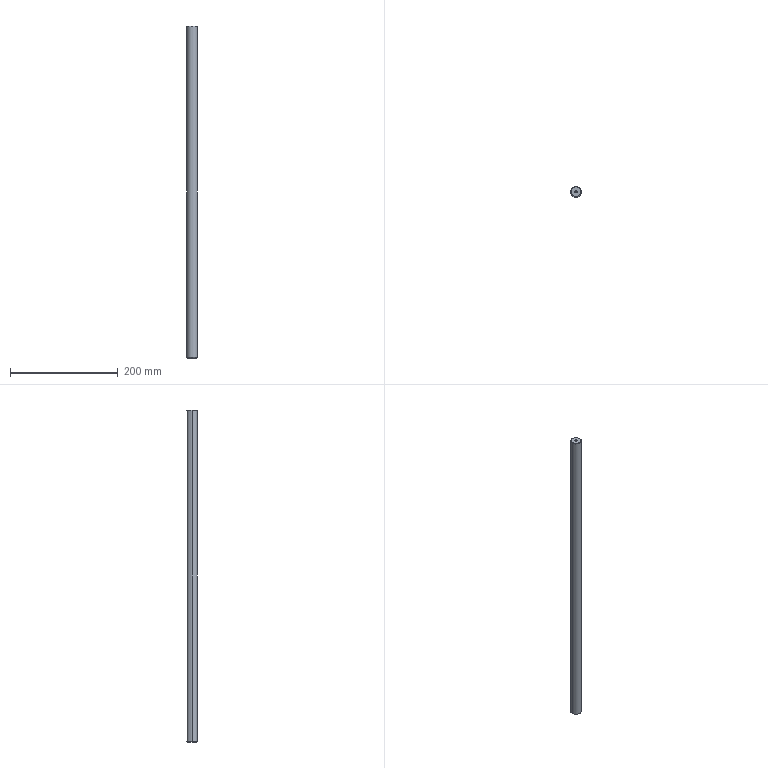Part | STEP file | Guide shaft 2 | 1 solid | 12 faces | box 20 x 20 x 616 mm | volume 193311 mm3 | cone 6 | cylinder 4 | plane 2 | commonest cylinder face diameters 4.2 x2 20 x2
STEP:
#1=CARTESIAN_POINT('',(0.,0.,0.));
#2=DIRECTION('',(0.,0.,1.));
#3=DIRECTION('',(1.,0.,0.));
#4=AXIS2_PLACEMENT_3D('',#1,#2,#3);
#5=CARTESIAN_POINT('',(2.1,0.,605.6));
#6=VERTEX_POINT('',#5);
#7=CARTESIAN_POINT('',(2.1,0.,616.));
#8=VERTEX_POINT('',#7);
#9=CARTESIAN_POINT('',(2.1,0.,616.));
#10=DIRECTION('',(0.,0.,1.));
#11=VECTOR('',#10,1.);
#12=LINE('',#9,#11);
#13=CARTESIAN_POINT('',(0.,0.,616.));
#14=DIRECTION('',(0.,0.,1.));
#15=DIRECTION('',(1.,0.,0.));
#16=AXIS2_PLACEMENT_3D('',#13,#14,#15);
#17=CYLINDRICAL_SURFACE('',#16,2.1);
#18=CARTESIAN_POINT('',(6.283,0.));
#19=DIRECTION('',(0.,1.));
#20=VECTOR('',#19,1.);
#21=LINE('',#18,#20);
#22=(GEOMETRIC_REPRESENTATION_CONTEXT(2)PARAMETRIC_REPRESENTATION_CONTEXT()REPRESENTATION_CONTEXT('',''));
#23=DEFINITIONAL_REPRESENTATION('',(#21),#22);
#24=PCURVE('',#17,#23);
#25=CARTESIAN_POINT('',(0.,0.,616.));
#26=DIRECTION('',(0.,0.,1.));
#27=DIRECTION('',(1.,0.,0.));
#28=AXIS2_PLACEMENT_3D('',#25,#26,#27);
#29=CYLINDRICAL_SURFACE('',#28,2.1);
#30=CARTESIAN_POINT('',(0.,0.));
#31=DIRECTION('',(0.,1.));
#32=VECTOR('',#31,1.);
#33=LINE('',#30,#32);
#34=(GEOMETRIC_REPRESENTATION_CONTEXT(2)PARAMETRIC_REPRESENTATION_CONTEXT()REPRESENTATION_CONTEXT('',''));
#35=DEFINITIONAL_REPRESENTATION('',(#33),#34);
#36=PCURVE('',#29,#35);
#37=SURFACE_CURVE('',#12,(#24,#36),.PCURVE_S1.);
#38=EDGE_CURVE('',#6,#8,#37,.T.);
#39=ORIENTED_EDGE('',*,*,#38,.T.);
#40=CARTESIAN_POINT('',(-2.1,0.,616.));
#41=VERTEX_POINT('',#40);
#42=CARTESIAN_POINT('',(0.,0.,616.));
#43=DIRECTION('',(0.,0.,1.));
#44=DIRECTION('',(1.,0.,0.));
#45=AXIS2_PLACEMENT_3D('',#42,#43,#44);
#46=CIRCLE('',#45,2.1);
#47=CARTESIAN_POINT('',(0.,0.));
#48=DIRECTION('',(1.,0.));
#49=VECTOR('',#48,1.);
#50=LINE('',#47,#49);
#51=(GEOMETRIC_REPRESENTATION_CONTEXT(2)PARAMETRIC_REPRESENTATION_CONTEXT()REPRESENTATION_CONTEXT('',''));
#52=DEFINITIONAL_REPRESENTATION('',(#50),#51);
#53=PCURVE('',#17,#52);
#54=CARTESIAN_POINT('',(0.,0.,616.));
#55=DIRECTION('',(0.,0.,1.));
#56=DIRECTION('',(1.,0.,0.));
#57=AXIS2_PLACEMENT_3D('',#54,#55,#56);
#58=PLANE('',#57);
#59=CARTESIAN_POINT('',(0.,0.));
#60=DIRECTION('',(1.,0.));
#61=AXIS2_PLACEMENT_2D('',#59,#60);
#62=CIRCLE('',#61,2.1);
#63=(GEOMETRIC_REPRESENTATION_CONTEXT(2)PARAMETRIC_REPRESENTATION_CONTEXT()REPRESENTATION_CONTEXT('',''));
#64=DEFINITIONAL_REPRESENTATION('',(#62),#63);
#65=PCURVE('',#58,#64);
#66=SURFACE_CURVE('',#46,(#53,#65),.PCURVE_S1.);
#67=EDGE_CURVE('',#41,#8,#66,.T.);
#68=ORIENTED_EDGE('',*,*,#67,.F.);
#69=CARTESIAN_POINT('',(-2.1,0.,605.6));
#70=VERTEX_POINT('',#69);
#71=CARTESIAN_POINT('',(-2.1,0.,616.));
#72=DIRECTION('',(0.,0.,1.));
#73=VECTOR('',#72,1.);
#74=LINE('',#71,#73);
#75=CARTESIAN_POINT('',(3.142,0.));
#76=DIRECTION('',(0.,1.));
#77=VECTOR('',#76,1.);
#78=LINE('',#75,#77);
#79=(GEOMETRIC_REPRESENTATION_CONTEXT(2)PARAMETRIC_REPRESENTATION_CONTEXT()REPRESENTATION_CONTEXT('',''));
#80=DEFINITIONAL_REPRESENTATION('',(#78),#79);
#81=PCURVE('',#17,#80);
#82=CARTESIAN_POINT('',(3.142,0.));
#83=DIRECTION('',(0.,1.));
#84=VECTOR('',#83,1.);
#85=LINE('',#82,#84);
#86=(GEOMETRIC_REPRESENTATION_CONTEXT(2)PARAMETRIC_REPRESENTATION_CONTEXT()REPRESENTATION_CONTEXT('',''));
#87=DEFINITIONAL_REPRESENTATION('',(#85),#86);
#88=PCURVE('',#29,#87);
#89=SURFACE_CURVE('',#74,(#81,#88),.PCURVE_S1.);
#90=EDGE_CURVE('',#70,#41,#89,.T.);
#91=ORIENTED_EDGE('',*,*,#90,.F.);
#92=CARTESIAN_POINT('',(0.,0.,605.6));
#93=DIRECTION('',(0.,0.,1.));
#94=DIRECTION('',(1.,0.,0.));
#95=AXIS2_PLACEMENT_3D('',#92,#93,#94);
#96=CIRCLE('',#95,2.1);
#97=CARTESIAN_POINT('',(0.,-10.4));
#98=DIRECTION('',(1.,0.));
#99=VECTOR('',#98,1.);
#100=LINE('',#97,#99);
#101=(GEOMETRIC_REPRESENTATION_CONTEXT(2)PARAMETRIC_REPRESENTATION_CONTEXT()REPRESENTATION_CONTEXT('',''));
#102=DEFINITIONAL_REPRESENTATION('',(#100),#101);
#103=PCURVE('',#17,#102);
#104=CARTESIAN_POINT('',(0.,0.,605.6));
#105=DIRECTION('',(0.,0.,1.));
#106=DIRECTION('',(1.,0.,0.));
#107=AXIS2_PLACEMENT_3D('',#104,#105,#106);
#108=CONICAL_SURFACE('',#107,2.1,1.03);
#109=CARTESIAN_POINT('',(0.,0.));
#110=DIRECTION('',(1.,0.));
#111=VECTOR('',#110,1.);
#112=LINE('',#109,#111);
#113=(GEOMETRIC_REPRESENTATION_CONTEXT(2)PARAMETRIC_REPRESENTATION_CONTEXT()REPRESENTATION_CONTEXT('',''));
#114=DEFINITIONAL_REPRESENTATION('',(#112),#113);
#115=PCURVE('',#108,#114);
#116=SURFACE_CURVE('',#96,(#103,#115),.PCURVE_S1.);
#117=EDGE_CURVE('',#70,#6,#116,.T.);
#118=ORIENTED_EDGE('',*,*,#117,.T.);
#119=EDGE_LOOP('',(#39,#68,#91,#118));
#120=FACE_BOUND('',#119,.F.);
#121=ADVANCED_FACE('',(#120),#17,.F.);
#122=ORIENTED_EDGE('',*,*,#117,.F.);
#123=CARTESIAN_POINT('',(0.,0.,604.338));
#124=VERTEX_POINT('',#123);
#125=CARTESIAN_POINT('',(-2.1,0.,605.6));
#126=DIRECTION('',(-0.8572,0.,0.515));
#127=VECTOR('',#126,1.);
#128=LINE('',#125,#127);
#129=CARTESIAN_POINT('',(3.142,0.));
#130=DIRECTION('',(0.,1.));
#131=VECTOR('',#130,1.);
#132=LINE('',#129,#131);
#133=(GEOMETRIC_REPRESENTATION_CONTEXT(2)PARAMETRIC_REPRESENTATION_CONTEXT()REPRESENTATION_CONTEXT('',''));
#134=DEFINITIONAL_REPRESENTATION('',(#132),#133);
#135=PCURVE('',#108,#134);
#136=CARTESIAN_POINT('',(0.,0.,605.6));
#137=DIRECTION('',(0.,0.,1.));
#138=DIRECTION('',(1.,0.,0.));
#139=AXIS2_PLACEMENT_3D('',#136,#137,#138);
#140=CONICAL_SURFACE('',#139,2.1,1.03);
#141=CARTESIAN_POINT('',(3.142,0.));
#142=DIRECTION('',(0.,1.));
#143=VECTOR('',#142,1.);
#144=LINE('',#141,#143);
#145=(GEOMETRIC_REPRESENTATION_CONTEXT(2)PARAMETRIC_REPRESENTATION_CONTEXT()REPRESENTATION_CONTEXT('',''));
#146=DEFINITIONAL_REPRESENTATION('',(#144),#145);
#147=PCURVE('',#140,#146);
#148=SURFACE_CURVE('',#128,(#135,#147),.PCURVE_S1.);
#149=EDGE_CURVE('',#124,#70,#148,.T.);
#150=ORIENTED_EDGE('',*,*,#149,.F.);
#151=CARTESIAN_POINT('',(2.1,0.,605.6));
#152=DIRECTION('',(0.8572,0.,0.515));
#153=VECTOR('',#152,1.);
#154=LINE('',#151,#153);
#155=CARTESIAN_POINT('',(6.283,0.));
#156=DIRECTION('',(0.,1.));
#157=VECTOR('',#156,1.);
#158=LINE('',#155,#157);
#159=(GEOMETRIC_REPRESENTATION_CONTEXT(2)PARAMETRIC_REPRESENTATION_CONTEXT()REPRESENTATION_CONTEXT('',''));
#160=DEFINITIONAL_REPRESENTATION('',(#158),#159);
#161=PCURVE('',#108,#160);
#162=CARTESIAN_POINT('',(0.,0.));
#163=DIRECTION('',(0.,1.));
#164=VECTOR('',#163,1.);
#165=LINE('',#162,#164);
#166=(GEOMETRIC_REPRESENTATION_CONTEXT(2)PARAMETRIC_REPRESENTATION_CONTEXT()REPRESENTATION_CONTEXT('',''));
#167=DEFINITIONAL_REPRESENTATION('',(#165),#166);
#168=PCURVE('',#140,#167);
#169=SURFACE_CURVE('',#154,(#161,#168),.PCURVE_S1.);
#170=EDGE_CURVE('',#124,#6,#169,.T.);
#171=ORIENTED_EDGE('',*,*,#170,.T.);
#172=EDGE_LOOP('',(#122,#150,#171));
#173=FACE_BOUND('',#172,.F.);
#174=ADVANCED_FACE('',(#173),#108,.F.);
#175=CARTESIAN_POINT('',(9.,0.,616.));
#176=VERTEX_POINT('',#175);
#177=CARTESIAN_POINT('',(-9.,0.,616.));
#178=VERTEX_POINT('',#177);
#179=CARTESIAN_POINT('',(0.,0.,616.));
#180=DIRECTION('',(0.,0.,1.));
#181=DIRECTION('',(1.,0.,0.));
#182=AXIS2_PLACEMENT_3D('',#179,#180,#181);
#183=CIRCLE('',#182,9.);
#184=CARTESIAN_POINT('',(0.,0.,616.));
#185=DIRECTION('',(0.,0.,-1.));
#186=DIRECTION('',(-1.,0.,0.));
#187=AXIS2_PLACEMENT_3D('',#184,#185,#186);
#188=CONICAL_SURFACE('',#187,9.,0.7854);
#189=CARTESIAN_POINT('',(3.142,0.));
#190=DIRECTION('',(-1.,0.));
#191=VECTOR('',#190,1.);
#192=LINE('',#189,#191);
#193=(GEOMETRIC_REPRESENTATION_CONTEXT(2)PARAMETRIC_REPRESENTATION_CONTEXT()REPRESENTATION_CONTEXT('',''));
#194=DEFINITIONAL_REPRESENTATION('',(#192),#193);
#195=PCURVE('',#188,#194);
#196=CARTESIAN_POINT('',(0.,0.));
#197=DIRECTION('',(1.,0.));
#198=AXIS2_PLACEMENT_2D('',#196,#197);
#199=CIRCLE('',#198,9.);
#200=(GEOMETRIC_REPRESENTATION_CONTEXT(2)PARAMETRIC_REPRESENTATION_CONTEXT()REPRESENTATION_CONTEXT('',''));
#201=DEFINITIONAL_REPRESENTATION('',(#199),#200);
#202=PCURVE('',#58,#201);
#203=SURFACE_CURVE('',#183,(#195,#202),.PCURVE_S1.);
#204=EDGE_CURVE('',#176,#178,#203,.T.);
#205=ORIENTED_EDGE('',*,*,#204,.F.);
#206=CARTESIAN_POINT('',(10.,0.,615.));
#207=VERTEX_POINT('',#206);
#208=CARTESIAN_POINT('',(9.,0.,616.));
#209=DIRECTION('',(0.7071,0.,-0.7071));
#210=VECTOR('',#209,1.);
#211=LINE('',#208,#210);
#212=CARTESIAN_POINT('',(3.142,0.));
#213=DIRECTION('',(0.,1.));
#214=VECTOR('',#213,1.);
#215=LINE('',#212,#214);
#216=(GEOMETRIC_REPRESENTATION_CONTEXT(2)PARAMETRIC_REPRESENTATION_CONTEXT()REPRESENTATION_CONTEXT('',''));
#217=DEFINITIONAL_REPRESENTATION('',(#215),#216);
#218=PCURVE('',#188,#217);
#219=CARTESIAN_POINT('',(0.,0.,616.));
#220=DIRECTION('',(0.,0.,-1.));
#221=DIRECTION('',(-1.,0.,0.));
#222=AXIS2_PLACEMENT_3D('',#219,#220,#221);
#223=CONICAL_SURFACE('',#222,9.,0.7854);
#224=CARTESIAN_POINT('',(3.142,0.));
#225=DIRECTION('',(0.,1.));
#226=VECTOR('',#225,1.);
#227=LINE('',#224,#226);
#228=(GEOMETRIC_REPRESENTATION_CONTEXT(2)PARAMETRIC_REPRESENTATION_CONTEXT()REPRESENTATION_CONTEXT('',''));
#229=DEFINITIONAL_REPRESENTATION('',(#227),#228);
#230=PCURVE('',#223,#229);
#231=SURFACE_CURVE('',#211,(#218,#230),.PCURVE_S1.);
#232=EDGE_CURVE('',#176,#207,#231,.T.);
#233=ORIENTED_EDGE('',*,*,#232,.T.);
#234=CARTESIAN_POINT('',(-10.,0.,615.));
#235=VERTEX_POINT('',#234);
#236=CARTESIAN_POINT('',(0.,0.,615.));
#237=DIRECTION('',(0.,0.,-1.));
#238=DIRECTION('',(1.,0.,0.));
#239=AXIS2_PLACEMENT_3D('',#236,#237,#238);
#240=CIRCLE('',#239,10.);
#241=CARTESIAN_POINT('',(-3.142,1.));
#242=DIRECTION('',(1.,0.));
#243=VECTOR('',#242,1.);
#244=LINE('',#241,#243);
#245=(GEOMETRIC_REPRESENTATION_CONTEXT(2)PARAMETRIC_REPRESENTATION_CONTEXT()REPRESENTATION_CONTEXT('',''));
#246=DEFINITIONAL_REPRESENTATION('',(#244),#245);
#247=PCURVE('',#188,#246);
#248=CARTESIAN_POINT('',(0.,0.,616.));
#249=DIRECTION('',(0.,0.,-1.));
#250=DIRECTION('',(-1.,0.,0.));
#251=AXIS2_PLACEMENT_3D('',#248,#249,#250);
#252=CYLINDRICAL_SURFACE('',#251,10.);
#253=CARTESIAN_POINT('',(-3.142,1.));
#254=DIRECTION('',(1.,0.));
#255=VECTOR('',#254,1.);
#256=LINE('',#253,#255);
#257=(GEOMETRIC_REPRESENTATION_CONTEXT(2)PARAMETRIC_REPRESENTATION_CONTEXT()REPRESENTATION_CONTEXT('',''));
#258=DEFINITIONAL_REPRESENTATION('',(#256),#257);
#259=PCURVE('',#252,#258);
#260=SURFACE_CURVE('',#240,(#247,#259),.PCURVE_S1.);
#261=EDGE_CURVE('',#235,#207,#260,.T.);
#262=ORIENTED_EDGE('',*,*,#261,.F.);
#263=CARTESIAN_POINT('',(-9.,0.,616.));
#264=DIRECTION('',(-0.7071,0.,-0.7071));
#265=VECTOR('',#264,1.);
#266=LINE('',#263,#265);
#267=CARTESIAN_POINT('',(0.,0.));
#268=DIRECTION('',(0.,1.));
#269=VECTOR('',#268,1.);
#270=LINE('',#267,#269);
#271=(GEOMETRIC_REPRESENTATION_CONTEXT(2)PARAMETRIC_REPRESENTATION_CONTEXT()REPRESENTATION_CONTEXT('',''));
#272=DEFINITIONAL_REPRESENTATION('',(#270),#271);
#273=PCURVE('',#188,#272);
#274=CARTESIAN_POINT('',(6.283,0.));
#275=DIRECTION('',(0.,1.));
#276=VECTOR('',#275,1.);
#277=LINE('',#274,#276);
#278=(GEOMETRIC_REPRESENTATION_CONTEXT(2)PARAMETRIC_REPRESENTATION_CONTEXT()REPRESENTATION_CONTEXT('',''));
#279=DEFINITIONAL_REPRESENTATION('',(#277),#278);
#280=PCURVE('',#223,#279);
#281=SURFACE_CURVE('',#266,(#273,#280),.PCURVE_S1.);
#282=EDGE_CURVE('',#178,#235,#281,.T.);
#283=ORIENTED_EDGE('',*,*,#282,.F.);
#284=EDGE_LOOP('',(#205,#233,#262,#283));
#285=FACE_BOUND('',#284,.T.);
#286=ADVANCED_FACE('',(#285),#188,.T.);
#287=CARTESIAN_POINT('',(-9.,0.,0.));
#288=VERTEX_POINT('',#287);
#289=CARTESIAN_POINT('',(9.,0.,0.));
#290=VERTEX_POINT('',#289);
#291=CARTESIAN_POINT('',(0.,0.,0.));
#292=DIRECTION('',(0.,0.,-1.));
#293=DIRECTION('',(1.,0.,0.));
#294=AXIS2_PLACEMENT_3D('',#291,#292,#293);
#295=CIRCLE('',#294,9.);
#296=CARTESIAN_POINT('',(0.,0.,1.));
#297=DIRECTION('',(0.,0.,1.));
#298=DIRECTION('',(1.,0.,0.));
#299=AXIS2_PLACEMENT_3D('',#296,#297,#298);
#300=CONICAL_SURFACE('',#299,10.,0.7854);
#301=CARTESIAN_POINT('',(6.283,-1.));
#302=DIRECTION('',(-1.,0.));
#303=VECTOR('',#302,1.);
#304=LINE('',#301,#303);
#305=(GEOMETRIC_REPRESENTATION_CONTEXT(2)PARAMETRIC_REPRESENTATION_CONTEXT()REPRESENTATION_CONTEXT('',''));
#306=DEFINITIONAL_REPRESENTATION('',(#304),#305);
#307=PCURVE('',#300,#306);
#308=CARTESIAN_POINT('',(0.,0.,0.));
#309=DIRECTION('',(0.,0.,1.));
#310=DIRECTION('',(1.,0.,0.));
#311=AXIS2_PLACEMENT_3D('',#308,#309,#310);
#312=PLANE('',#311);
#313=CARTESIAN_POINT('',(9.,0.));
#314=CARTESIAN_POINT('',(9.,-15.588));
#315=CARTESIAN_POINT('',(-4.5,-7.794));
#316=CARTESIAN_POINT('',(-18.,0.));
#317=CARTESIAN_POINT('',(-4.5,7.794));
#318=CARTESIAN_POINT('',(9.,15.588));
#319=CARTESIAN_POINT('',(9.,0.));
#320=(BOUNDED_CURVE()B_SPLINE_CURVE(2,(#313,#314,#315,#316,#317,#318,#319),.UNSPECIFIED.,.T.,.F.)B_SPLINE_CURVE_WITH_KNOTS((1,2,2,2,2,1),(-2.094,0.,2.094,4.189,6.283,8.378),.UNSPECIFIED.)CURVE()GEOMETRIC_REPRESENTATION_ITEM()RATIONAL_B_SPLINE_CURVE((1.,0.5,1.,0.5,1.,0.5,1.))REPRESENTATION_ITEM(''));
#321=(GEOMETRIC_REPRESENTATION_CONTEXT(2)PARAMETRIC_REPRESENTATION_CONTEXT()REPRESENTATION_CONTEXT('',''));
#322=DEFINITIONAL_REPRESENTATION('',(#320),#321);
#323=PCURVE('',#312,#322);
#324=SURFACE_CURVE('',#295,(#307,#323),.PCURVE_S1.);
#325=EDGE_CURVE('',#288,#290,#324,.T.);
#326=ORIENTED_EDGE('',*,*,#325,.F.);
#327=CARTESIAN_POINT('',(-10.,0.,1.));
#328=VERTEX_POINT('',#327);
#329=CARTESIAN_POINT('',(-10.,0.,1.));
#330=DIRECTION('',(-0.7071,0.,0.7071));
#331=VECTOR('',#330,1.);
#332=LINE('',#329,#331);
#333=CARTESIAN_POINT('',(3.142,0.));
#334=DIRECTION('',(0.,1.));
#335=VECTOR('',#334,1.);
#336=LINE('',#333,#335);
#337=(GEOMETRIC_REPRESENTATION_CONTEXT(2)PARAMETRIC_REPRESENTATION_CONTEXT()REPRESENTATION_CONTEXT('',''));
#338=DEFINITIONAL_REPRESENTATION('',(#336),#337);
#339=PCURVE('',#300,#338);
#340=CARTESIAN_POINT('',(0.,0.,1.));
#341=DIRECTION('',(0.,0.,1.));
#342=DIRECTION('',(1.,0.,0.));
#343=AXIS2_PLACEMENT_3D('',#340,#341,#342);
#344=CONICAL_SURFACE('',#343,10.,0.7854);
#345=CARTESIAN_POINT('',(3.142,0.));
#346=DIRECTION('',(0.,1.));
#347=VECTOR('',#346,1.);
#348=LINE('',#345,#347);
#349=(GEOMETRIC_REPRESENTATION_CONTEXT(2)PARAMETRIC_REPRESENTATION_CONTEXT()REPRESENTATION_CONTEXT('',''));
#350=DEFINITIONAL_REPRESENTATION('',(#348),#349);
#351=PCURVE('',#344,#350);
#352=SURFACE_CURVE('',#332,(#339,#351),.PCURVE_S1.);
#353=EDGE_CURVE('',#288,#328,#352,.T.);
#354=ORIENTED_EDGE('',*,*,#353,.T.);
#355=CARTESIAN_POINT('',(10.,0.,1.));
#356=VERTEX_POINT('',#355);
#357=CARTESIAN_POINT('',(0.,0.,1.));
#358=DIRECTION('',(0.,0.,1.));
#359=DIRECTION('',(1.,0.,0.));
#360=AXIS2_PLACEMENT_3D('',#357,#358,#359);
#361=CIRCLE('',#360,10.);
#362=CARTESIAN_POINT('',(0.,0.));
#363=DIRECTION('',(1.,0.));
#364=VECTOR('',#363,1.);
#365=LINE('',#362,#364);
#366=(GEOMETRIC_REPRESENTATION_CONTEXT(2)PARAMETRIC_REPRESENTATION_CONTEXT()REPRESENTATION_CONTEXT('',''));
#367=DEFINITIONAL_REPRESENTATION('',(#365),#366);
#368=PCURVE('',#300,#367);
#369=CARTESIAN_POINT('',(3.142,615.));
#370=DIRECTION('',(-1.,0.));
#371=VECTOR('',#370,1.);
#372=LINE('',#369,#371);
#373=(GEOMETRIC_REPRESENTATION_CONTEXT(2)PARAMETRIC_REPRESENTATION_CONTEXT()REPRESENTATION_CONTEXT('',''));
#374=DEFINITIONAL_REPRESENTATION('',(#372),#373);
#375=PCURVE('',#252,#374);
#376=SURFACE_CURVE('',#361,(#368,#375),.PCURVE_S1.);
#377=EDGE_CURVE('',#356,#328,#376,.T.);
#378=ORIENTED_EDGE('',*,*,#377,.F.);
#379=CARTESIAN_POINT('',(10.,0.,1.));
#380=DIRECTION('',(0.7071,0.,0.7071));
#381=VECTOR('',#380,1.);
#382=LINE('',#379,#381);
#383=CARTESIAN_POINT('',(0.,0.));
#384=DIRECTION('',(0.,1.));
#385=VECTOR('',#384,1.);
#386=LINE('',#383,#385);
#387=(GEOMETRIC_REPRESENTATION_CONTEXT(2)PARAMETRIC_REPRESENTATION_CONTEXT()REPRESENTATION_CONTEXT('',''));
#388=DEFINITIONAL_REPRESENTATION('',(#386),#387);
#389=PCURVE('',#300,#388);
#390=CARTESIAN_POINT('',(6.283,0.));
#391=DIRECTION('',(0.,1.));
#392=VECTOR('',#391,1.);
#393=LINE('',#390,#392);
#394=(GEOMETRIC_REPRESENTATION_CONTEXT(2)PARAMETRIC_REPRESENTATION_CONTEXT()REPRESENTATION_CONTEXT('',''));
#395=DEFINITIONAL_REPRESENTATION('',(#393),#394);
#396=PCURVE('',#344,#395);
#397=SURFACE_CURVE('',#382,(#389,#396),.PCURVE_S1.);
#398=EDGE_CURVE('',#290,#356,#397,.T.);
#399=ORIENTED_EDGE('',*,*,#398,.F.);
#400=EDGE_LOOP('',(#326,#354,#378,#399));
#401=FACE_BOUND('',#400,.T.);
#402=ADVANCED_FACE('',(#401),#300,.T.);
#403=ORIENTED_EDGE('',*,*,#261,.T.);
#404=CARTESIAN_POINT('',(10.,0.,616.));
#405=DIRECTION('',(0.,0.,-1.));
#406=VECTOR('',#405,1.);
#407=LINE('',#404,#406);
#408=CARTESIAN_POINT('',(3.142,0.));
#409=DIRECTION('',(0.,1.));
#410=VECTOR('',#409,1.);
#411=LINE('',#408,#410);
#412=(GEOMETRIC_REPRESENTATION_CONTEXT(2)PARAMETRIC_REPRESENTATION_CONTEXT()REPRESENTATION_CONTEXT('',''));
#413=DEFINITIONAL_REPRESENTATION('',(#411),#412);
#414=PCURVE('',#252,#413);
#415=CARTESIAN_POINT('',(0.,0.,616.));
#416=DIRECTION('',(0.,0.,-1.));
#417=DIRECTION('',(-1.,0.,0.));
#418=AXIS2_PLACEMENT_3D('',#415,#416,#417);
#419=CYLINDRICAL_SURFACE('',#418,10.);
#420=CARTESIAN_POINT('',(3.142,0.));
#421=DIRECTION('',(0.,1.));
#422=VECTOR('',#421,1.);
#423=LINE('',#420,#422);
#424=(GEOMETRIC_REPRESENTATION_CONTEXT(2)PARAMETRIC_REPRESENTATION_CONTEXT()REPRESENTATION_CONTEXT('',''));
#425=DEFINITIONAL_REPRESENTATION('',(#423),#424);
#426=PCURVE('',#419,#425);
#427=SURFACE_CURVE('',#407,(#414,#426),.PCURVE_S1.);
#428=EDGE_CURVE('',#207,#356,#427,.T.);
#429=ORIENTED_EDGE('',*,*,#428,.T.);
#430=ORIENTED_EDGE('',*,*,#377,.T.);
#431=CARTESIAN_POINT('',(-10.,0.,616.));
#432=DIRECTION('',(0.,0.,-1.));
#433=VECTOR('',#432,1.);
#434=LINE('',#431,#433);
#435=CARTESIAN_POINT('',(0.,0.));
#436=DIRECTION('',(0.,1.));
#437=VECTOR('',#436,1.);
#438=LINE('',#435,#437);
#439=(GEOMETRIC_REPRESENTATION_CONTEXT(2)PARAMETRIC_REPRESENTATION_CONTEXT()REPRESENTATION_CONTEXT('',''));
#440=DEFINITIONAL_REPRESENTATION('',(#438),#439);
#441=PCURVE('',#252,#440);
#442=CARTESIAN_POINT('',(6.283,0.));
#443=DIRECTION('',(0.,1.));
#444=VECTOR('',#443,1.);
#445=LINE('',#442,#444);
#446=(GEOMETRIC_REPRESENTATION_CONTEXT(2)PARAMETRIC_REPRESENTATION_CONTEXT()REPRESENTATION_CONTEXT('',''));
#447=DEFINITIONAL_REPRESENTATION('',(#445),#446);
#448=PCURVE('',#419,#447);
#449=SURFACE_CURVE('',#434,(#441,#448),.PCURVE_S1.);
#450=EDGE_CURVE('',#235,#328,#449,.T.);
#451=ORIENTED_EDGE('',*,*,#450,.F.);
#452=EDGE_LOOP('',(#403,#429,#430,#451));
#453=FACE_BOUND('',#452,.T.);
#454=ADVANCED_FACE('',(#453),#252,.T.);
#455=ORIENTED_EDGE('',*,*,#428,.F.);
#456=CARTESIAN_POINT('',(0.,0.,615.));
#457=DIRECTION('',(0.,0.,-1.));
#458=DIRECTION('',(1.,0.,0.));
#459=AXIS2_PLACEMENT_3D('',#456,#457,#458);
#460=CIRCLE('',#459,10.);
#461=CARTESIAN_POINT('',(3.142,1.));
#462=DIRECTION('',(1.,0.));
#463=VECTOR('',#462,1.);
#464=LINE('',#461,#463);
#465=(GEOMETRIC_REPRESENTATION_CONTEXT(2)PARAMETRIC_REPRESENTATION_CONTEXT()REPRESENTATION_CONTEXT('',''));
#466=DEFINITIONAL_REPRESENTATION('',(#464),#465);
#467=PCURVE('',#419,#466);
#468=CARTESIAN_POINT('',(3.142,1.));
#469=DIRECTION('',(1.,0.));
#470=VECTOR('',#469,1.);
#471=LINE('',#468,#470);
#472=(GEOMETRIC_REPRESENTATION_CONTEXT(2)PARAMETRIC_REPRESENTATION_CONTEXT()REPRESENTATION_CONTEXT('',''));
#473=DEFINITIONAL_REPRESENTATION('',(#471),#472);
#474=PCURVE('',#223,#473);
#475=SURFACE_CURVE('',#460,(#467,#474),.PCURVE_S1.);
#476=EDGE_CURVE('',#207,#235,#475,.T.);
#477=ORIENTED_EDGE('',*,*,#476,.T.);
#478=ORIENTED_EDGE('',*,*,#450,.T.);
#479=CARTESIAN_POINT('',(0.,0.,1.));
#480=DIRECTION('',(0.,0.,1.));
#481=DIRECTION('',(1.,0.,0.));
#482=AXIS2_PLACEMENT_3D('',#479,#480,#481);
#483=CIRCLE('',#482,10.);
#484=CARTESIAN_POINT('',(9.425,615.));
#485=DIRECTION('',(-1.,0.));
#486=VECTOR('',#485,1.);
#487=LINE('',#484,#486);
#488=(GEOMETRIC_REPRESENTATION_CONTEXT(2)PARAMETRIC_REPRESENTATION_CONTEXT()REPRESENTATION_CONTEXT('',''));
#489=DEFINITIONAL_REPRESENTATION('',(#487),#488);
#490=PCURVE('',#419,#489);
#491=CARTESIAN_POINT('',(0.,0.));
#492=DIRECTION('',(1.,0.));
#493=VECTOR('',#492,1.);
#494=LINE('',#491,#493);
#495=(GEOMETRIC_REPRESENTATION_CONTEXT(2)PARAMETRIC_REPRESENTATION_CONTEXT()REPRESENTATION_CONTEXT('',''));
#496=DEFINITIONAL_REPRESENTATION('',(#494),#495);
#497=PCURVE('',#344,#496);
#498=SURFACE_CURVE('',#483,(#490,#497),.PCURVE_S1.);
#499=EDGE_CURVE('',#328,#356,#498,.T.);
#500=ORIENTED_EDGE('',*,*,#499,.T.);
#501=EDGE_LOOP('',(#455,#477,#478,#500));
#502=FACE_BOUND('',#501,.T.);
#503=ADVANCED_FACE('',(#502),#419,.T.);
#504=CARTESIAN_POINT('',(0.,0.,616.));
#505=DIRECTION('',(0.,0.,1.));
#506=DIRECTION('',(1.,0.,0.));
#507=AXIS2_PLACEMENT_3D('',#504,#505,#506);
#508=CIRCLE('',#507,2.1);
#509=CARTESIAN_POINT('',(0.,0.));
#510=DIRECTION('',(1.,0.));
#511=AXIS2_PLACEMENT_2D('',#509,#510);
#512=CIRCLE('',#511,2.1);
#513=(GEOMETRIC_REPRESENTATION_CONTEXT(2)PARAMETRIC_REPRESENTATION_CONTEXT()REPRESENTATION_CONTEXT('',''));
#514=DEFINITIONAL_REPRESENTATION('',(#512),#513);
#515=PCURVE('',#58,#514);
#516=CARTESIAN_POINT('',(0.,0.));
#517=DIRECTION('',(1.,0.));
#518=VECTOR('',#517,1.);
#519=LINE('',#516,#518);
#520=(GEOMETRIC_REPRESENTATION_CONTEXT(2)PARAMETRIC_REPRESENTATION_CONTEXT()REPRESENTATION_CONTEXT('',''));
#521=DEFINITIONAL_REPRESENTATION('',(#519),#520);
#522=PCURVE('',#29,#521);
#523=SURFACE_CURVE('',#508,(#515,#522),.PCURVE_S1.);
#524=EDGE_CURVE('',#8,#41,#523,.T.);
#525=ORIENTED_EDGE('',*,*,#524,.F.);
#526=ORIENTED_EDGE('',*,*,#67,.F.);
#527=EDGE_LOOP('',(#525,#526));
#528=FACE_BOUND('',#527,.T.);
#529=CARTESIAN_POINT('',(0.,0.,616.));
#530=DIRECTION('',(0.,0.,1.));
#531=DIRECTION('',(1.,0.,0.));
#532=AXIS2_PLACEMENT_3D('',#529,#530,#531);
#533=CIRCLE('',#532,9.);
#534=CARTESIAN_POINT('',(0.,0.));
#535=DIRECTION('',(1.,0.));
#536=AXIS2_PLACEMENT_2D('',#534,#535);
#537=CIRCLE('',#536,9.);
#538=(GEOMETRIC_REPRESENTATION_CONTEXT(2)PARAMETRIC_REPRESENTATION_CONTEXT()REPRESENTATION_CONTEXT('',''));
#539=DEFINITIONAL_REPRESENTATION('',(#537),#538);
#540=PCURVE('',#58,#539);
#541=CARTESIAN_POINT('',(9.425,0.));
#542=DIRECTION('',(-1.,0.));
#543=VECTOR('',#542,1.);
#544=LINE('',#541,#543);
#545=(GEOMETRIC_REPRESENTATION_CONTEXT(2)PARAMETRIC_REPRESENTATION_CONTEXT()REPRESENTATION_CONTEXT('',''));
#546=DEFINITIONAL_REPRESENTATION('',(#544),#545);
#547=PCURVE('',#223,#546);
#548=SURFACE_CURVE('',#533,(#540,#547),.PCURVE_S1.);
#549=EDGE_CURVE('',#178,#176,#548,.T.);
#550=ORIENTED_EDGE('',*,*,#549,.T.);
#551=ORIENTED_EDGE('',*,*,#204,.T.);
#552=EDGE_LOOP('',(#550,#551));
#553=FACE_BOUND('',#552,.T.);
#554=ADVANCED_FACE('',(#528,#553),#58,.T.);
#555=CARTESIAN_POINT('',(0.,0.,0.));
#556=DIRECTION('',(0.,0.,-1.));
#557=DIRECTION('',(1.,0.,0.));
#558=AXIS2_PLACEMENT_3D('',#555,#556,#557);
#559=CIRCLE('',#558,9.);
#560=CARTESIAN_POINT('',(9.,0.));
#561=CARTESIAN_POINT('',(9.,-15.588));
#562=CARTESIAN_POINT('',(-4.5,-7.794));
#563=CARTESIAN_POINT('',(-18.,0.));
#564=CARTESIAN_POINT('',(-4.5,7.794));
#565=CARTESIAN_POINT('',(9.,15.588));
#566=CARTESIAN_POINT('',(9.,0.));
#567=(BOUNDED_CURVE()B_SPLINE_CURVE(2,(#560,#561,#562,#563,#564,#565,#566),.UNSPECIFIED.,.T.,.F.)B_SPLINE_CURVE_WITH_KNOTS((1,2,2,2,2,1),(-2.094,0.,2.094,4.189,6.283,8.378),.UNSPECIFIED.)CURVE()GEOMETRIC_REPRESENTATION_ITEM()RATIONAL_B_SPLINE_CURVE((1.,0.5,1.,0.5,1.,0.5,1.))REPRESENTATION_ITEM(''));
#568=(GEOMETRIC_REPRESENTATION_CONTEXT(2)PARAMETRIC_REPRESENTATION_CONTEXT()REPRESENTATION_CONTEXT('',''));
#569=DEFINITIONAL_REPRESENTATION('',(#567),#568);
#570=PCURVE('',#312,#569);
#571=CARTESIAN_POINT('',(6.283,-1.));
#572=DIRECTION('',(-1.,0.));
#573=VECTOR('',#572,1.);
#574=LINE('',#571,#573);
#575=(GEOMETRIC_REPRESENTATION_CONTEXT(2)PARAMETRIC_REPRESENTATION_CONTEXT()REPRESENTATION_CONTEXT('',''));
#576=DEFINITIONAL_REPRESENTATION('',(#574),#575);
#577=PCURVE('',#344,#576);
#578=SURFACE_CURVE('',#559,(#570,#577),.PCURVE_S1.);
#579=EDGE_CURVE('',#290,#288,#578,.T.);
#580=ORIENTED_EDGE('',*,*,#579,.T.);
#581=ORIENTED_EDGE('',*,*,#325,.T.);
#582=EDGE_LOOP('',(#580,#581));
#583=FACE_BOUND('',#582,.T.);
#584=ADVANCED_FACE('',(#583),#312,.F.);
#585=ORIENTED_EDGE('',*,*,#353,.F.);
#586=ORIENTED_EDGE('',*,*,#579,.F.);
#587=ORIENTED_EDGE('',*,*,#398,.T.);
#588=ORIENTED_EDGE('',*,*,#499,.F.);
#589=EDGE_LOOP('',(#585,#586,#587,#588));
#590=FACE_BOUND('',#589,.T.);
#591=ADVANCED_FACE('',(#590),#344,.T.);
#592=ORIENTED_EDGE('',*,*,#232,.F.);
#593=ORIENTED_EDGE('',*,*,#549,.F.);
#594=ORIENTED_EDGE('',*,*,#282,.T.);
#595=ORIENTED_EDGE('',*,*,#476,.F.);
#596=EDGE_LOOP('',(#592,#593,#594,#595));
#597=FACE_BOUND('',#596,.T.);
#598=ADVANCED_FACE('',(#597),#223,.T.);
#599=CARTESIAN_POINT('',(0.,0.,605.6));
#600=DIRECTION('',(0.,0.,1.));
#601=DIRECTION('',(1.,0.,0.));
#602=AXIS2_PLACEMENT_3D('',#599,#600,#601);
#603=CIRCLE('',#602,2.1);
#604=CARTESIAN_POINT('',(0.,0.));
#605=DIRECTION('',(1.,0.));
#606=VECTOR('',#605,1.);
#607=LINE('',#604,#606);
#608=(GEOMETRIC_REPRESENTATION_CONTEXT(2)PARAMETRIC_REPRESENTATION_CONTEXT()REPRESENTATION_CONTEXT('',''));
#609=DEFINITIONAL_REPRESENTATION('',(#607),#608);
#610=PCURVE('',#140,#609);
#611=CARTESIAN_POINT('',(0.,-10.4));
#612=DIRECTION('',(1.,0.));
#613=VECTOR('',#612,1.);
#614=LINE('',#611,#613);
#615=(GEOMETRIC_REPRESENTATION_CONTEXT(2)PARAMETRIC_REPRESENTATION_CONTEXT()REPRESENTATION_CONTEXT('',''));
#616=DEFINITIONAL_REPRESENTATION('',(#614),#615);
#617=PCURVE('',#29,#616);
#618=SURFACE_CURVE('',#603,(#610,#617),.PCURVE_S1.);
#619=EDGE_CURVE('',#6,#70,#618,.T.);
#620=ORIENTED_EDGE('',*,*,#619,.F.);
#621=ORIENTED_EDGE('',*,*,#170,.F.);
#622=ORIENTED_EDGE('',*,*,#149,.T.);
#623=EDGE_LOOP('',(#620,#621,#622));
#624=FACE_BOUND('',#623,.F.);
#625=ADVANCED_FACE('',(#624),#140,.F.);
#626=ORIENTED_EDGE('',*,*,#524,.F.);
#627=ORIENTED_EDGE('',*,*,#38,.F.);
#628=ORIENTED_EDGE('',*,*,#619,.T.);
#629=ORIENTED_EDGE('',*,*,#90,.T.);
#630=EDGE_LOOP('',(#626,#627,#628,#629));
#631=FACE_BOUND('',#630,.F.);
#632=ADVANCED_FACE('',(#631),#29,.F.);
#633=CLOSED_SHELL('',(#121,#174,#286,#402,#454,#503,#554,#584,#591,#598,#625,#632));
#634=MANIFOLD_SOLID_BREP('',#633);
#635=(LENGTH_UNIT()NAMED_UNIT(*)SI_UNIT(.MILLI.,.METRE.));
#636=UNCERTAINTY_MEASURE_WITH_UNIT(LENGTH_MEASURE(0.0000001),#635,'','');
#637=(NAMED_UNIT(*)PLANE_ANGLE_UNIT()SI_UNIT($,.RADIAN.));
#638=(NAMED_UNIT(*)SI_UNIT($,.STERADIAN.)SOLID_ANGLE_UNIT());
#639=(GEOMETRIC_REPRESENTATION_CONTEXT(3)GLOBAL_UNCERTAINTY_ASSIGNED_CONTEXT((#636))GLOBAL_UNIT_ASSIGNED_CONTEXT((#635,#637,#638))REPRESENTATION_CONTEXT('',''));
#640=ADVANCED_BREP_SHAPE_REPRESENTATION('',(#4,#634),#639);